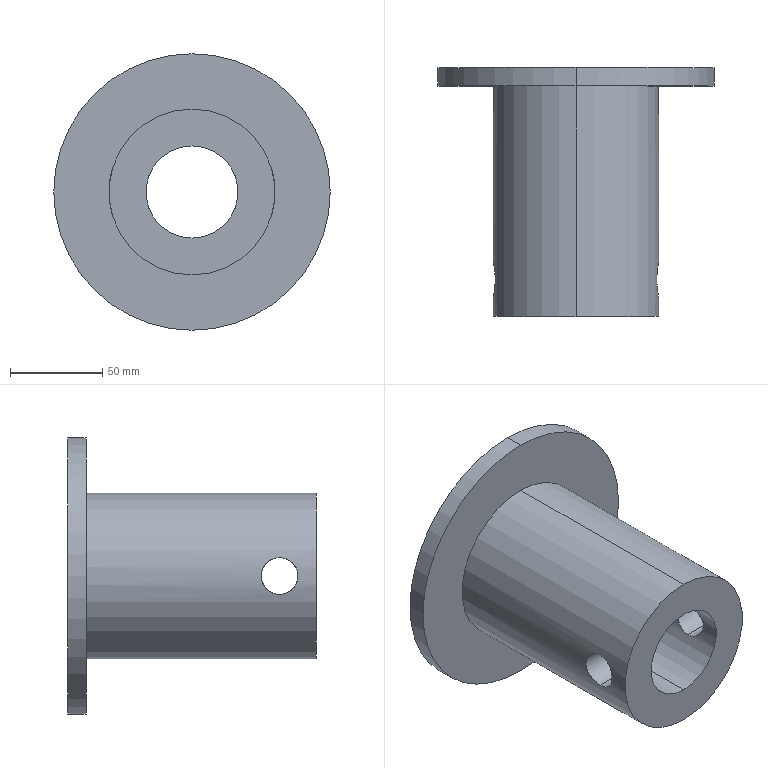Part | SolidWorks | features ICE 2, Extrusion 1 | 1 solid | 13 faces | box 150 x 135 x 150 mm | volume 694147 mm3 | cylinder 10 | plane 3 | commonest cylinder face diameters 20 x4 50 x2 90 x2 150 x2
STEP:
#1=CARTESIAN_POINT('',(-43.875,-105.,10.));
#2=VERTEX_POINT('',#1);
#3=CARTESIAN_POINT('',(-43.875,-105.,-10.));
#4=VERTEX_POINT('',#3);
#5=CARTESIAN_POINT('',(-43.875,-105.,10.));
#6=CARTESIAN_POINT('',(-43.875,-105.654,10.));
#7=CARTESIAN_POINT('',(-43.889,-106.305,9.937));
#8=CARTESIAN_POINT('',(-43.947,-107.602,9.678));
#9=CARTESIAN_POINT('',(-43.989,-108.229,9.487));
#10=CARTESIAN_POINT('',(-44.068,-109.132,9.112));
#11=CARTESIAN_POINT('',(-44.097,-109.427,8.973));
#12=CARTESIAN_POINT('',(-44.158,-110.005,8.663));
#13=CARTESIAN_POINT('',(-44.192,-110.289,8.493));
#14=CARTESIAN_POINT('',(-44.294,-111.104,7.948));
#15=CARTESIAN_POINT('',(-44.367,-111.606,7.536));
#16=CARTESIAN_POINT('',(-44.477,-112.298,6.845));
#17=CARTESIAN_POINT('',(-44.514,-112.519,6.601));
#18=CARTESIAN_POINT('',(-44.586,-112.936,6.094));
#19=CARTESIAN_POINT('',(-44.621,-113.13,5.831));
#20=CARTESIAN_POINT('',(-44.722,-113.673,5.02));
#21=CARTESIAN_POINT('',(-44.784,-113.981,4.447));
#22=CARTESIAN_POINT('',(-44.862,-114.36,3.536));
#23=CARTESIAN_POINT('',(-44.885,-114.472,3.224));
#24=CARTESIAN_POINT('',(-44.926,-114.662,2.598));
#25=CARTESIAN_POINT('',(-44.961,-114.821,1.965));
#26=CARTESIAN_POINT('',(-44.982,-114.918,1.318));
#27=CARTESIAN_POINT('',(-44.996,-114.983,0.6657));
#28=CARTESIAN_POINT('',(-45.,-115.,0.3341));
#29=CARTESIAN_POINT('',(-45.,-115.,-0.6558));
#30=CARTESIAN_POINT('',(-44.986,-114.936,-1.306));
#31=CARTESIAN_POINT('',(-44.93,-114.681,-2.589));
#32=CARTESIAN_POINT('',(-44.888,-114.488,-3.227));
#33=CARTESIAN_POINT('',(-44.785,-113.987,-4.434));
#34=CARTESIAN_POINT('',(-44.724,-113.68,-5.008));
#35=CARTESIAN_POINT('',(-44.622,-113.135,-5.825));
#36=CARTESIAN_POINT('',(-44.587,-112.938,-6.091));
#37=CARTESIAN_POINT('',(-44.515,-112.523,-6.596));
#38=CARTESIAN_POINT('',(-44.478,-112.305,-6.837));
#39=CARTESIAN_POINT('',(-44.405,-111.846,-7.297));
#40=CARTESIAN_POINT('',(-44.369,-111.605,-7.515));
#41=CARTESIAN_POINT('',(-44.296,-111.102,-7.929));
#42=CARTESIAN_POINT('',(-44.261,-110.838,-8.126));
#43=CARTESIAN_POINT('',(-44.158,-110.019,-8.674));
#44=CARTESIAN_POINT('',(-44.095,-109.445,-8.982));
#45=CARTESIAN_POINT('',(-44.017,-108.543,-9.357));
#46=CARTESIAN_POINT('',(-43.993,-108.235,-9.468));
#47=CARTESIAN_POINT('',(-43.951,-107.606,-9.66));
#48=CARTESIAN_POINT('',(-43.933,-107.284,-9.741));
#49=CARTESIAN_POINT('',(-43.89,-106.317,-9.935));
#50=CARTESIAN_POINT('',(-43.875,-105.663,-10.));
#51=CARTESIAN_POINT('',(-43.875,-105.,-10.));
#52=B_SPLINE_CURVE_WITH_KNOTS('',3,(#5,#6,#7,#8,#9,#10,#11,#12,#13,#14,#15,#16,#17,#18,#19,#20,#21,#22,#23,#24,#25,#26,#27,#28,#29,#30,#31,#32,#33,#34,#35,#36,#37,#38,#39,#40,#41,#42,#43,#44,#45,#46,#47,#48,#49,#50,#51),.UNSPECIFIED.,.F.,.F.,(4,2,2,2,2,2,2,2,2,2,1,2,2,2,2,2,2,2,2,2,2,2,2,4),(0.03136,0.03332,0.03528,0.03626,0.03724,0.0392,0.04018,0.04116,0.04312,0.0441,0.04508,0.04606,0.04704,0.049,0.05096,0.05292,0.0539,0.05488,0.05586,0.05684,0.0588,0.05978,0.06076,0.06272),.UNSPECIFIED.);
#53=EDGE_CURVE('',#2,#4,#52,.T.);
#54=ORIENTED_EDGE('',*,*,#53,.F.);
#55=CARTESIAN_POINT('',(-22.913,-105.,10.));
#56=VERTEX_POINT('',#55);
#57=CARTESIAN_POINT('',(-75.,-105.,10.));
#58=DIRECTION('',(1.,0.,0.));
#59=VECTOR('',#58,1000.);
#60=LINE('',#57,#59);
#61=EDGE_CURVE('',#2,#56,#60,.T.);
#62=ORIENTED_EDGE('',*,*,#61,.T.);
#63=CARTESIAN_POINT('',(-22.913,-105.,-10.));
#64=VERTEX_POINT('',#63);
#65=CARTESIAN_POINT('',(-22.913,-105.,10.));
#66=CARTESIAN_POINT('',(-22.913,-105.329,10.));
#67=CARTESIAN_POINT('',(-22.92,-105.658,9.984));
#68=CARTESIAN_POINT('',(-22.948,-106.316,9.918));
#69=CARTESIAN_POINT('',(-22.97,-106.648,9.869));
#70=CARTESIAN_POINT('',(-23.053,-107.619,9.674));
#71=CARTESIAN_POINT('',(-23.134,-108.244,9.482));
#72=CARTESIAN_POINT('',(-23.284,-109.15,9.104));
#73=CARTESIAN_POINT('',(-23.339,-109.449,8.962));
#74=CARTESIAN_POINT('',(-23.456,-110.024,8.652));
#75=CARTESIAN_POINT('',(-23.517,-110.302,8.485));
#76=CARTESIAN_POINT('',(-23.707,-111.108,7.944));
#77=CARTESIAN_POINT('',(-23.843,-111.61,7.532));
#78=CARTESIAN_POINT('',(-24.115,-112.532,6.61));
#79=CARTESIAN_POINT('',(-24.248,-112.942,6.111));
#80=CARTESIAN_POINT('',(-24.432,-113.482,5.306));
#81=CARTESIAN_POINT('',(-24.491,-113.65,5.028));
#82=CARTESIAN_POINT('',(-24.602,-113.96,4.452));
#83=CARTESIAN_POINT('',(-24.655,-114.103,4.153));
#84=CARTESIAN_POINT('',(-24.796,-114.481,3.247));
#85=CARTESIAN_POINT('',(-24.87,-114.672,2.623));
#86=CARTESIAN_POINT('',(-24.947,-114.867,1.656));
#87=CARTESIAN_POINT('',(-24.967,-114.917,1.327));
#88=CARTESIAN_POINT('',(-24.993,-114.983,0.6643));
#89=CARTESIAN_POINT('',(-25.,-115.,0.3339));
#90=CARTESIAN_POINT('',(-25.,-115.,-0.6544));
#91=CARTESIAN_POINT('',(-24.974,-114.936,-1.31));
#92=CARTESIAN_POINT('',(-24.897,-114.741,-2.287));
#93=CARTESIAN_POINT('',(-24.866,-114.659,-2.609));
#94=CARTESIAN_POINT('',(-24.792,-114.467,-3.237));
#95=CARTESIAN_POINT('',(-24.749,-114.357,-3.544));
#96=CARTESIAN_POINT('',(-24.656,-114.106,-4.147));
#97=CARTESIAN_POINT('',(-24.604,-113.965,-4.442));
#98=CARTESIAN_POINT('',(-24.493,-113.656,-5.019));
#99=CARTESIAN_POINT('',(-24.433,-113.486,-5.301));
#100=CARTESIAN_POINT('',(-24.248,-112.942,-6.111));
#101=CARTESIAN_POINT('',(-24.115,-112.532,-6.609));
#102=CARTESIAN_POINT('',(-23.912,-111.845,-7.298));
#103=CARTESIAN_POINT('',(-23.844,-111.602,-7.518));
#104=CARTESIAN_POINT('',(-23.71,-111.1,-7.931));
#105=CARTESIAN_POINT('',(-23.644,-110.841,-8.124));
#106=CARTESIAN_POINT('',(-23.454,-110.036,-8.664));
#107=CARTESIAN_POINT('',(-23.336,-109.466,-8.972));
#108=CARTESIAN_POINT('',(-23.185,-108.554,-9.353));
#109=CARTESIAN_POINT('',(-23.139,-108.244,-9.465));
#110=CARTESIAN_POINT('',(-23.06,-107.617,-9.657));
#111=CARTESIAN_POINT('',(-23.026,-107.299,-9.738));
#112=CARTESIAN_POINT('',(-22.97,-106.655,-9.867));
#113=CARTESIAN_POINT('',(-22.949,-106.329,-9.917));
#114=CARTESIAN_POINT('',(-22.92,-105.669,-9.983));
#115=CARTESIAN_POINT('',(-22.913,-105.334,-10.));
#116=CARTESIAN_POINT('',(-22.913,-105.,-10.));
#117=B_SPLINE_CURVE_WITH_KNOTS('',3,(#65,#66,#67,#68,#69,#70,#71,#72,#73,#74,#75,#76,#77,#78,#79,#80,#81,#82,#83,#84,#85,#86,#87,#88,#89,#90,#91,#92,#93,#94,#95,#96,#97,#98,#99,#100,#101,#102,#103,#104,#105,#106,#107,#108,#109,#110,#111,#112,#113,#114,#115,#116),.UNSPECIFIED.,.F.,.F.,(4,2,2,2,2,2,2,2,2,2,2,2,2,2,2,2,2,2,2,2,2,2,2,2,2,4),(0.0316,0.03258,0.03357,0.03554,0.03653,0.03752,0.03949,0.04146,0.04245,0.04344,0.04541,0.04639,0.04738,0.04935,0.05034,0.05133,0.05231,0.0533,0.05527,0.05626,0.05725,0.05922,0.06021,0.06119,0.06218,0.06317),.UNSPECIFIED.);
#118=EDGE_CURVE('',#56,#64,#117,.T.);
#119=ORIENTED_EDGE('',*,*,#118,.T.);
#120=CARTESIAN_POINT('',(-75.,-105.,-10.));
#121=DIRECTION('',(1.,0.,0.));
#122=VECTOR('',#121,1000.);
#123=LINE('',#120,#122);
#124=EDGE_CURVE('',#4,#64,#123,.T.);
#125=ORIENTED_EDGE('',*,*,#124,.F.);
#126=EDGE_LOOP('',(#54,#62,#119,#125));
#127=FACE_OUTER_BOUND('',#126,.T.);
#128=CARTESIAN_POINT('',(-75.,-105.,0.));
#129=DIRECTION('',(1.,0.,0.));
#130=DIRECTION('',(0.,0.,-1.));
#131=AXIS2_PLACEMENT_3D('',#128,#129,#130);
#132=CYLINDRICAL_SURFACE('',#131,10.);
#133=ADVANCED_FACE('',(#127),#132,.F.);
#134=CARTESIAN_POINT('',(22.913,-105.,-10.));
#135=VERTEX_POINT('',#134);
#136=CARTESIAN_POINT('',(22.913,-105.,10.));
#137=VERTEX_POINT('',#136);
#138=CARTESIAN_POINT('',(22.913,-105.,-10.));
#139=CARTESIAN_POINT('',(22.913,-105.668,-10.));
#140=CARTESIAN_POINT('',(22.942,-106.324,-9.934));
#141=CARTESIAN_POINT('',(23.025,-107.29,-9.74));
#142=CARTESIAN_POINT('',(23.059,-107.608,-9.659));
#143=CARTESIAN_POINT('',(23.139,-108.24,-9.466));
#144=CARTESIAN_POINT('',(23.185,-108.552,-9.354));
#145=CARTESIAN_POINT('',(23.335,-109.457,-8.976));
#146=CARTESIAN_POINT('',(23.452,-110.028,-8.668));
#147=CARTESIAN_POINT('',(23.644,-110.839,-8.125));
#148=CARTESIAN_POINT('',(23.71,-111.103,-7.929));
#149=CARTESIAN_POINT('',(23.844,-111.604,-7.516));
#150=CARTESIAN_POINT('',(23.912,-111.843,-7.299));
#151=CARTESIAN_POINT('',(24.114,-112.528,-6.615));
#152=CARTESIAN_POINT('',(24.247,-112.941,-6.113));
#153=CARTESIAN_POINT('',(24.496,-113.67,-5.026));
#154=CARTESIAN_POINT('',(24.608,-113.977,-4.454));
#155=CARTESIAN_POINT('',(24.748,-114.353,-3.553));
#156=CARTESIAN_POINT('',(24.791,-114.465,-3.245));
#157=CARTESIAN_POINT('',(24.865,-114.658,-2.615));
#158=CARTESIAN_POINT('',(24.897,-114.74,-2.291));
#159=CARTESIAN_POINT('',(24.974,-114.935,-1.32));
#160=CARTESIAN_POINT('',(25.,-115.,-0.6657));
#161=CARTESIAN_POINT('',(25.,-115.,0.3251));
#162=CARTESIAN_POINT('',(24.994,-114.984,0.6588));
#163=CARTESIAN_POINT('',(24.967,-114.918,1.321));
#164=CARTESIAN_POINT('',(24.948,-114.869,1.648));
#165=CARTESIAN_POINT('',(24.871,-114.674,2.615));
#166=CARTESIAN_POINT('',(24.796,-114.483,3.243));
#167=CARTESIAN_POINT('',(24.606,-113.973,4.463));
#168=CARTESIAN_POINT('',(24.494,-113.664,5.036));
#169=CARTESIAN_POINT('',(24.309,-113.122,5.843));
#170=CARTESIAN_POINT('',(24.245,-112.928,6.104));
#171=CARTESIAN_POINT('',(24.112,-112.513,6.608));
#172=CARTESIAN_POINT('',(24.045,-112.293,6.849));
#173=CARTESIAN_POINT('',(23.842,-111.606,7.535));
#174=CARTESIAN_POINT('',(23.707,-111.108,7.945));
#175=CARTESIAN_POINT('',(23.516,-110.298,8.488));
#176=CARTESIAN_POINT('',(23.454,-110.016,8.657));
#177=CARTESIAN_POINT('',(23.337,-109.44,8.966));
#178=CARTESIAN_POINT('',(23.283,-109.146,9.106));
#179=CARTESIAN_POINT('',(23.134,-108.245,9.481));
#180=CARTESIAN_POINT('',(23.053,-107.621,9.673));
#181=CARTESIAN_POINT('',(22.969,-106.644,9.87));
#182=CARTESIAN_POINT('',(22.948,-106.314,9.919));
#183=CARTESIAN_POINT('',(22.92,-105.658,9.984));
#184=CARTESIAN_POINT('',(22.913,-105.329,10.));
#185=CARTESIAN_POINT('',(22.913,-105.,10.));
#186=B_SPLINE_CURVE_WITH_KNOTS('',3,(#138,#139,#140,#141,#142,#143,#144,#145,#146,#147,#148,#149,#150,#151,#152,#153,#154,#155,#156,#157,#158,#159,#160,#161,#162,#163,#164,#165,#166,#167,#168,#169,#170,#171,#172,#173,#174,#175,#176,#177,#178,#179,#180,#181,#182,#183,#184,#185),.UNSPECIFIED.,.F.,.F.,(4,2,2,2,2,2,2,2,2,2,2,2,2,2,2,2,2,2,2,2,2,2,2,4),(0.,0.001975,0.002962,0.00395,0.005924,0.006912,0.007899,0.009874,0.01185,0.01284,0.01382,0.0158,0.01679,0.01777,0.01975,0.02172,0.02271,0.0237,0.02567,0.02666,0.02765,0.02962,0.03061,0.0316),.UNSPECIFIED.);
#187=EDGE_CURVE('',#135,#137,#186,.T.);
#188=ORIENTED_EDGE('',*,*,#187,.T.);
#189=CARTESIAN_POINT('',(43.875,-105.,10.));
#190=VERTEX_POINT('',#189);
#191=CARTESIAN_POINT('',(-75.,-105.,10.));
#192=DIRECTION('',(1.,0.,0.));
#193=VECTOR('',#192,1000.);
#194=LINE('',#191,#193);
#195=EDGE_CURVE('',#137,#190,#194,.T.);
#196=ORIENTED_EDGE('',*,*,#195,.T.);
#197=CARTESIAN_POINT('',(43.875,-105.,-10.));
#198=VERTEX_POINT('',#197);
#199=CARTESIAN_POINT('',(43.875,-105.,-10.));
#200=CARTESIAN_POINT('',(43.875,-105.663,-10.));
#201=CARTESIAN_POINT('',(43.89,-106.314,-9.935));
#202=CARTESIAN_POINT('',(43.933,-107.275,-9.743));
#203=CARTESIAN_POINT('',(43.95,-107.593,-9.664));
#204=CARTESIAN_POINT('',(43.992,-108.222,-9.472));
#205=CARTESIAN_POINT('',(44.016,-108.534,-9.36));
#206=CARTESIAN_POINT('',(44.095,-109.442,-8.983));
#207=CARTESIAN_POINT('',(44.157,-110.015,-8.676));
#208=CARTESIAN_POINT('',(44.26,-110.829,-8.132));
#209=CARTESIAN_POINT('',(44.295,-111.094,-7.935));
#210=CARTESIAN_POINT('',(44.368,-111.601,-7.519));
#211=CARTESIAN_POINT('',(44.405,-111.843,-7.299));
#212=CARTESIAN_POINT('',(44.514,-112.532,-6.61));
#213=CARTESIAN_POINT('',(44.587,-112.945,-6.108));
#214=CARTESIAN_POINT('',(44.689,-113.494,-5.288));
#215=CARTESIAN_POINT('',(44.722,-113.663,-5.005));
#216=CARTESIAN_POINT('',(44.782,-113.971,-4.43));
#217=CARTESIAN_POINT('',(44.811,-114.111,-4.135));
#218=CARTESIAN_POINT('',(44.862,-114.36,-3.534));
#219=CARTESIAN_POINT('',(44.885,-114.471,-3.227));
#220=CARTESIAN_POINT('',(44.926,-114.662,-2.6));
#221=CARTESIAN_POINT('',(44.943,-114.743,-2.278));
#222=CARTESIAN_POINT('',(44.986,-114.936,-1.309));
#223=CARTESIAN_POINT('',(45.,-115.,-0.6585));
#224=CARTESIAN_POINT('',(45.,-115.,0.6506));
#225=CARTESIAN_POINT('',(44.985,-114.935,1.316));
#226=CARTESIAN_POINT('',(44.929,-114.678,2.6));
#227=CARTESIAN_POINT('',(44.888,-114.489,3.224));
#228=CARTESIAN_POINT('',(44.811,-114.111,4.134));
#229=CARTESIAN_POINT('',(44.782,-113.969,4.434));
#230=CARTESIAN_POINT('',(44.721,-113.66,5.011));
#231=CARTESIAN_POINT('',(44.689,-113.492,5.29));
#232=CARTESIAN_POINT('',(44.621,-113.131,5.831));
#233=CARTESIAN_POINT('',(44.586,-112.937,6.092));
#234=CARTESIAN_POINT('',(44.515,-112.523,6.596));
#235=CARTESIAN_POINT('',(44.478,-112.302,6.84));
#236=CARTESIAN_POINT('',(44.367,-111.605,7.536));
#237=CARTESIAN_POINT('',(44.294,-111.103,7.949));
#238=CARTESIAN_POINT('',(44.192,-110.292,8.491));
#239=CARTESIAN_POINT('',(44.159,-110.012,8.66));
#240=CARTESIAN_POINT('',(44.097,-109.432,8.97));
#241=CARTESIAN_POINT('',(44.068,-109.134,9.112));
#242=CARTESIAN_POINT('',(43.989,-108.228,9.487));
#243=CARTESIAN_POINT('',(43.947,-107.604,9.677));
#244=CARTESIAN_POINT('',(43.904,-106.639,9.87));
#245=CARTESIAN_POINT('',(43.893,-106.311,9.919));
#246=CARTESIAN_POINT('',(43.878,-105.654,9.984));
#247=CARTESIAN_POINT('',(43.875,-105.327,10.));
#248=CARTESIAN_POINT('',(43.875,-105.,10.));
#249=B_SPLINE_CURVE_WITH_KNOTS('',3,(#199,#200,#201,#202,#203,#204,#205,#206,#207,#208,#209,#210,#211,#212,#213,#214,#215,#216,#217,#218,#219,#220,#221,#222,#223,#224,#225,#226,#227,#228,#229,#230,#231,#232,#233,#234,#235,#236,#237,#238,#239,#240,#241,#242,#243,#244,#245,#246,#247,#248),.UNSPECIFIED.,.F.,.F.,(4,2,2,2,2,2,2,2,2,2,2,2,2,2,2,2,2,2,2,2,2,2,2,2,4),(0.,0.00196,0.00294,0.00392,0.00588,0.006861,0.007841,0.009801,0.01078,0.01176,0.01274,0.01372,0.01568,0.01764,0.0196,0.02058,0.02156,0.02254,0.02352,0.02548,0.02646,0.02744,0.0294,0.03038,0.03136),.UNSPECIFIED.);
#250=EDGE_CURVE('',#198,#190,#249,.T.);
#251=ORIENTED_EDGE('',*,*,#250,.F.);
#252=CARTESIAN_POINT('',(-75.,-105.,-10.));
#253=DIRECTION('',(1.,0.,0.));
#254=VECTOR('',#253,1000.);
#255=LINE('',#252,#254);
#256=EDGE_CURVE('',#135,#198,#255,.T.);
#257=ORIENTED_EDGE('',*,*,#256,.F.);
#258=EDGE_LOOP('',(#188,#196,#251,#257));
#259=FACE_OUTER_BOUND('',#258,.T.);
#260=CARTESIAN_POINT('',(-75.,-105.,0.));
#261=DIRECTION('',(1.,0.,0.));
#262=DIRECTION('',(0.,0.,-1.));
#263=AXIS2_PLACEMENT_3D('',#260,#261,#262);
#264=CYLINDRICAL_SURFACE('',#263,10.);
#265=ADVANCED_FACE('',(#259),#264,.F.);
#266=ORIENTED_EDGE('',*,*,#250,.T.);
#267=CARTESIAN_POINT('',(43.875,-105.,10.));
#268=CARTESIAN_POINT('',(43.875,-104.346,10.));
#269=CARTESIAN_POINT('',(43.889,-103.695,9.937));
#270=CARTESIAN_POINT('',(43.947,-102.398,9.678));
#271=CARTESIAN_POINT('',(43.989,-101.771,9.487));
#272=CARTESIAN_POINT('',(44.068,-100.868,9.112));
#273=CARTESIAN_POINT('',(44.097,-100.573,8.973));
#274=CARTESIAN_POINT('',(44.158,-99.995,8.663));
#275=CARTESIAN_POINT('',(44.192,-99.711,8.493));
#276=CARTESIAN_POINT('',(44.294,-98.896,7.948));
#277=CARTESIAN_POINT('',(44.367,-98.394,7.536));
#278=CARTESIAN_POINT('',(44.477,-97.702,6.845));
#279=CARTESIAN_POINT('',(44.514,-97.481,6.601));
#280=CARTESIAN_POINT('',(44.586,-97.064,6.094));
#281=CARTESIAN_POINT('',(44.621,-96.87,5.831));
#282=CARTESIAN_POINT('',(44.722,-96.327,5.02));
#283=CARTESIAN_POINT('',(44.784,-96.019,4.447));
#284=CARTESIAN_POINT('',(44.862,-95.64,3.536));
#285=CARTESIAN_POINT('',(44.885,-95.528,3.224));
#286=CARTESIAN_POINT('',(44.926,-95.338,2.598));
#287=CARTESIAN_POINT('',(44.961,-95.179,1.965));
#288=CARTESIAN_POINT('',(44.982,-95.082,1.318));
#289=CARTESIAN_POINT('',(44.996,-95.017,0.6657));
#290=CARTESIAN_POINT('',(45.,-95.,0.3341));
#291=CARTESIAN_POINT('',(45.,-95.,-0.6558));
#292=CARTESIAN_POINT('',(44.986,-95.064,-1.306));
#293=CARTESIAN_POINT('',(44.93,-95.319,-2.589));
#294=CARTESIAN_POINT('',(44.888,-95.512,-3.227));
#295=CARTESIAN_POINT('',(44.785,-96.013,-4.434));
#296=CARTESIAN_POINT('',(44.724,-96.32,-5.008));
#297=CARTESIAN_POINT('',(44.622,-96.865,-5.825));
#298=CARTESIAN_POINT('',(44.587,-97.062,-6.091));
#299=CARTESIAN_POINT('',(44.515,-97.477,-6.596));
#300=CARTESIAN_POINT('',(44.478,-97.695,-6.837));
#301=CARTESIAN_POINT('',(44.405,-98.154,-7.297));
#302=CARTESIAN_POINT('',(44.369,-98.395,-7.515));
#303=CARTESIAN_POINT('',(44.296,-98.898,-7.929));
#304=CARTESIAN_POINT('',(44.261,-99.162,-8.126));
#305=CARTESIAN_POINT('',(44.158,-99.981,-8.674));
#306=CARTESIAN_POINT('',(44.095,-100.555,-8.982));
#307=CARTESIAN_POINT('',(44.017,-101.457,-9.357));
#308=CARTESIAN_POINT('',(43.993,-101.765,-9.468));
#309=CARTESIAN_POINT('',(43.951,-102.394,-9.66));
#310=CARTESIAN_POINT('',(43.933,-102.716,-9.741));
#311=CARTESIAN_POINT('',(43.89,-103.683,-9.935));
#312=CARTESIAN_POINT('',(43.875,-104.337,-10.));
#313=CARTESIAN_POINT('',(43.875,-105.,-10.));
#314=B_SPLINE_CURVE_WITH_KNOTS('',3,(#267,#268,#269,#270,#271,#272,#273,#274,#275,#276,#277,#278,#279,#280,#281,#282,#283,#284,#285,#286,#287,#288,#289,#290,#291,#292,#293,#294,#295,#296,#297,#298,#299,#300,#301,#302,#303,#304,#305,#306,#307,#308,#309,#310,#311,#312,#313),.UNSPECIFIED.,.F.,.F.,(4,2,2,2,2,2,2,2,2,2,1,2,2,2,2,2,2,2,2,2,2,2,2,4),(0.03136,0.03332,0.03528,0.03626,0.03724,0.0392,0.04018,0.04116,0.04312,0.0441,0.04508,0.04606,0.04704,0.049,0.05096,0.05292,0.0539,0.05488,0.05586,0.05684,0.0588,0.05978,0.06076,0.06272),.UNSPECIFIED.);
#315=EDGE_CURVE('',#190,#198,#314,.T.);
#316=ORIENTED_EDGE('',*,*,#315,.T.);
#317=EDGE_LOOP('',(#266,#316));
#318=FACE_BOUND('',#317,.T.);
#319=CARTESIAN_POINT('',(0.,-125.,-45.));
#320=VERTEX_POINT('',#319);
#321=CARTESIAN_POINT('',(0.,-125.,45.));
#322=VERTEX_POINT('',#321);
#323=CARTESIAN_POINT('',(0.,-125.,0.));
#324=DIRECTION('',(0.,-1.,0.));
#325=DIRECTION('',(0.,0.,-1.));
#326=AXIS2_PLACEMENT_3D('',#323,#324,#325);
#327=CIRCLE('',#326,45.);
#328=EDGE_CURVE('',#320,#322,#327,.T.);
#329=ORIENTED_EDGE('',*,*,#328,.F.);
#330=CARTESIAN_POINT('',(0.,0.,-45.));
#331=VERTEX_POINT('',#330);
#332=CARTESIAN_POINT('',(0.,-125.,-45.));
#333=DIRECTION('',(0.,1.,0.));
#334=VECTOR('',#333,1000.);
#335=LINE('',#332,#334);
#336=EDGE_CURVE('',#320,#331,#335,.T.);
#337=ORIENTED_EDGE('',*,*,#336,.T.);
#338=CARTESIAN_POINT('',(0.,0.,45.));
#339=VERTEX_POINT('',#338);
#340=CARTESIAN_POINT('',(0.,0.,0.));
#341=DIRECTION('',(0.,-1.,0.));
#342=DIRECTION('',(0.,0.,1.));
#343=AXIS2_PLACEMENT_3D('',#340,#341,#342);
#344=CIRCLE('',#343,45.);
#345=EDGE_CURVE('',#331,#339,#344,.T.);
#346=ORIENTED_EDGE('',*,*,#345,.T.);
#347=CARTESIAN_POINT('',(0.,-125.,45.));
#348=DIRECTION('',(0.,1.,0.));
#349=VECTOR('',#348,1000.);
#350=LINE('',#347,#349);
#351=EDGE_CURVE('',#322,#339,#350,.T.);
#352=ORIENTED_EDGE('',*,*,#351,.F.);
#353=EDGE_LOOP('',(#329,#337,#346,#352));
#354=FACE_OUTER_BOUND('',#353,.T.);
#355=CARTESIAN_POINT('',(0.,-125.,0.));
#356=DIRECTION('',(0.,1.,0.));
#357=DIRECTION('',(0.,0.,1.));
#358=AXIS2_PLACEMENT_3D('',#355,#356,#357);
#359=CYLINDRICAL_SURFACE('',#358,45.);
#360=ADVANCED_FACE('',(#318,#354),#359,.T.);
#361=CARTESIAN_POINT('',(-22.913,-105.,-10.));
#362=CARTESIAN_POINT('',(-22.913,-104.332,-10.));
#363=CARTESIAN_POINT('',(-22.942,-103.676,-9.934));
#364=CARTESIAN_POINT('',(-23.025,-102.71,-9.74));
#365=CARTESIAN_POINT('',(-23.059,-102.392,-9.659));
#366=CARTESIAN_POINT('',(-23.139,-101.76,-9.466));
#367=CARTESIAN_POINT('',(-23.185,-101.448,-9.354));
#368=CARTESIAN_POINT('',(-23.335,-100.543,-8.976));
#369=CARTESIAN_POINT('',(-23.452,-99.972,-8.668));
#370=CARTESIAN_POINT('',(-23.644,-99.161,-8.125));
#371=CARTESIAN_POINT('',(-23.71,-98.897,-7.929));
#372=CARTESIAN_POINT('',(-23.844,-98.396,-7.516));
#373=CARTESIAN_POINT('',(-23.912,-98.157,-7.299));
#374=CARTESIAN_POINT('',(-24.114,-97.472,-6.615));
#375=CARTESIAN_POINT('',(-24.247,-97.059,-6.113));
#376=CARTESIAN_POINT('',(-24.496,-96.33,-5.026));
#377=CARTESIAN_POINT('',(-24.608,-96.023,-4.454));
#378=CARTESIAN_POINT('',(-24.748,-95.647,-3.553));
#379=CARTESIAN_POINT('',(-24.791,-95.535,-3.245));
#380=CARTESIAN_POINT('',(-24.865,-95.342,-2.615));
#381=CARTESIAN_POINT('',(-24.897,-95.26,-2.291));
#382=CARTESIAN_POINT('',(-24.974,-95.065,-1.32));
#383=CARTESIAN_POINT('',(-25.,-95.,-0.6657));
#384=CARTESIAN_POINT('',(-25.,-95.,0.3251));
#385=CARTESIAN_POINT('',(-24.994,-95.016,0.6588));
#386=CARTESIAN_POINT('',(-24.967,-95.082,1.321));
#387=CARTESIAN_POINT('',(-24.948,-95.131,1.648));
#388=CARTESIAN_POINT('',(-24.871,-95.326,2.615));
#389=CARTESIAN_POINT('',(-24.796,-95.517,3.243));
#390=CARTESIAN_POINT('',(-24.606,-96.027,4.463));
#391=CARTESIAN_POINT('',(-24.494,-96.336,5.036));
#392=CARTESIAN_POINT('',(-24.309,-96.878,5.843));
#393=CARTESIAN_POINT('',(-24.245,-97.072,6.104));
#394=CARTESIAN_POINT('',(-24.112,-97.487,6.608));
#395=CARTESIAN_POINT('',(-24.045,-97.707,6.849));
#396=CARTESIAN_POINT('',(-23.842,-98.394,7.535));
#397=CARTESIAN_POINT('',(-23.707,-98.892,7.945));
#398=CARTESIAN_POINT('',(-23.516,-99.702,8.488));
#399=CARTESIAN_POINT('',(-23.454,-99.984,8.657));
#400=CARTESIAN_POINT('',(-23.337,-100.56,8.966));
#401=CARTESIAN_POINT('',(-23.283,-100.854,9.106));
#402=CARTESIAN_POINT('',(-23.134,-101.755,9.481));
#403=CARTESIAN_POINT('',(-23.053,-102.379,9.673));
#404=CARTESIAN_POINT('',(-22.969,-103.356,9.87));
#405=CARTESIAN_POINT('',(-22.948,-103.686,9.919));
#406=CARTESIAN_POINT('',(-22.92,-104.342,9.984));
#407=CARTESIAN_POINT('',(-22.913,-104.671,10.));
#408=CARTESIAN_POINT('',(-22.913,-105.,10.));
#409=B_SPLINE_CURVE_WITH_KNOTS('',3,(#361,#362,#363,#364,#365,#366,#367,#368,#369,#370,#371,#372,#373,#374,#375,#376,#377,#378,#379,#380,#381,#382,#383,#384,#385,#386,#387,#388,#389,#390,#391,#392,#393,#394,#395,#396,#397,#398,#399,#400,#401,#402,#403,#404,#405,#406,#407,#408),.UNSPECIFIED.,.F.,.F.,(4,2,2,2,2,2,2,2,2,2,2,2,2,2,2,2,2,2,2,2,2,2,2,4),(0.,0.001975,0.002962,0.00395,0.005924,0.006912,0.007899,0.009874,0.01185,0.01284,0.01382,0.0158,0.01679,0.01777,0.01975,0.02172,0.02271,0.0237,0.02567,0.02666,0.02765,0.02962,0.03061,0.0316),.UNSPECIFIED.);
#410=EDGE_CURVE('',#64,#56,#409,.T.);
#411=ORIENTED_EDGE('',*,*,#410,.F.);
#412=ORIENTED_EDGE('',*,*,#118,.F.);
#413=EDGE_LOOP('',(#411,#412));
#414=FACE_BOUND('',#413,.T.);
#415=CARTESIAN_POINT('',(0.,10.,-25.));
#416=VERTEX_POINT('',#415);
#417=CARTESIAN_POINT('',(0.,10.,25.));
#418=VERTEX_POINT('',#417);
#419=CARTESIAN_POINT('',(0.,10.,0.));
#420=DIRECTION('',(0.,1.,0.));
#421=DIRECTION('',(0.,0.,1.));
#422=AXIS2_PLACEMENT_3D('',#419,#420,#421);
#423=CIRCLE('',#422,25.);
#424=EDGE_CURVE('',#416,#418,#423,.T.);
#425=ORIENTED_EDGE('',*,*,#424,.T.);
#426=CARTESIAN_POINT('',(0.,-125.,25.));
#427=VERTEX_POINT('',#426);
#428=CARTESIAN_POINT('',(0.,10.,25.));
#429=DIRECTION('',(0.,-1.,0.));
#430=VECTOR('',#429,1000.);
#431=LINE('',#428,#430);
#432=EDGE_CURVE('',#418,#427,#431,.T.);
#433=ORIENTED_EDGE('',*,*,#432,.T.);
#434=CARTESIAN_POINT('',(0.,-125.,-25.));
#435=VERTEX_POINT('',#434);
#436=CARTESIAN_POINT('',(0.,-125.,0.));
#437=DIRECTION('',(0.,-1.,0.));
#438=DIRECTION('',(0.,0.,-1.));
#439=AXIS2_PLACEMENT_3D('',#436,#437,#438);
#440=CIRCLE('',#439,25.);
#441=EDGE_CURVE('',#427,#435,#440,.T.);
#442=ORIENTED_EDGE('',*,*,#441,.T.);
#443=CARTESIAN_POINT('',(0.,10.,-25.));
#444=DIRECTION('',(0.,-1.,0.));
#445=VECTOR('',#444,1000.);
#446=LINE('',#443,#445);
#447=EDGE_CURVE('',#416,#435,#446,.T.);
#448=ORIENTED_EDGE('',*,*,#447,.F.);
#449=EDGE_LOOP('',(#425,#433,#442,#448));
#450=FACE_OUTER_BOUND('',#449,.T.);
#451=CARTESIAN_POINT('',(0.,10.,0.));
#452=DIRECTION('',(0.,-1.,0.));
#453=DIRECTION('',(0.,0.,-1.));
#454=AXIS2_PLACEMENT_3D('',#451,#452,#453);
#455=CYLINDRICAL_SURFACE('',#454,25.);
#456=ADVANCED_FACE('',(#414,#450),#455,.F.);
#457=CARTESIAN_POINT('',(0.,10.,75.));
#458=VERTEX_POINT('',#457);
#459=CARTESIAN_POINT('',(0.,10.,-75.));
#460=VERTEX_POINT('',#459);
#461=CARTESIAN_POINT('',(0.,10.,0.));
#462=DIRECTION('',(0.,1.,0.));
#463=DIRECTION('',(0.,0.,1.));
#464=AXIS2_PLACEMENT_3D('',#461,#462,#463);
#465=CIRCLE('',#464,75.);
#466=EDGE_CURVE('',#458,#460,#465,.T.);
#467=ORIENTED_EDGE('',*,*,#466,.F.);
#468=CARTESIAN_POINT('',(0.,0.,75.));
#469=VERTEX_POINT('',#468);
#470=CARTESIAN_POINT('',(0.,10.,75.));
#471=DIRECTION('',(0.,-1.,0.));
#472=VECTOR('',#471,1000.);
#473=LINE('',#470,#472);
#474=EDGE_CURVE('',#458,#469,#473,.T.);
#475=ORIENTED_EDGE('',*,*,#474,.T.);
#476=CARTESIAN_POINT('',(0.,0.,-75.));
#477=VERTEX_POINT('',#476);
#478=CARTESIAN_POINT('',(0.,0.,0.));
#479=DIRECTION('',(0.,1.,0.));
#480=DIRECTION('',(0.,0.,1.));
#481=AXIS2_PLACEMENT_3D('',#478,#479,#480);
#482=CIRCLE('',#481,75.);
#483=EDGE_CURVE('',#469,#477,#482,.T.);
#484=ORIENTED_EDGE('',*,*,#483,.T.);
#485=CARTESIAN_POINT('',(0.,10.,-75.));
#486=DIRECTION('',(0.,-1.,0.));
#487=VECTOR('',#486,1000.);
#488=LINE('',#485,#487);
#489=EDGE_CURVE('',#460,#477,#488,.T.);
#490=ORIENTED_EDGE('',*,*,#489,.F.);
#491=EDGE_LOOP('',(#467,#475,#484,#490));
#492=FACE_OUTER_BOUND('',#491,.T.);
#493=CARTESIAN_POINT('',(0.,10.,0.));
#494=DIRECTION('',(0.,-1.,0.));
#495=DIRECTION('',(0.,0.,-1.));
#496=AXIS2_PLACEMENT_3D('',#493,#494,#495);
#497=CYLINDRICAL_SURFACE('',#496,75.);
#498=ADVANCED_FACE('',(#492),#497,.T.);
#499=CARTESIAN_POINT('',(0.,0.,0.));
#500=DIRECTION('',(0.,1.,0.));
#501=DIRECTION('',(0.,0.,1.));
#502=AXIS2_PLACEMENT_3D('',#499,#500,#501);
#503=CIRCLE('',#502,75.);
#504=EDGE_CURVE('',#477,#469,#503,.T.);
#505=ORIENTED_EDGE('',*,*,#504,.F.);
#506=ORIENTED_EDGE('',*,*,#483,.F.);
#507=EDGE_LOOP('',(#505,#506));
#508=FACE_OUTER_BOUND('',#507,.T.);
#509=CARTESIAN_POINT('',(0.,0.,0.));
#510=DIRECTION('',(0.,-1.,0.));
#511=DIRECTION('',(0.,0.,1.));
#512=AXIS2_PLACEMENT_3D('',#509,#510,#511);
#513=CIRCLE('',#512,45.);
#514=EDGE_CURVE('',#339,#331,#513,.T.);
#515=ORIENTED_EDGE('',*,*,#514,.F.);
#516=ORIENTED_EDGE('',*,*,#345,.F.);
#517=EDGE_LOOP('',(#515,#516));
#518=FACE_BOUND('',#517,.T.);
#519=CARTESIAN_POINT('',(0.,0.,0.));
#520=DIRECTION('',(0.,1.,0.));
#521=DIRECTION('',(0.,0.,1.));
#522=AXIS2_PLACEMENT_3D('',#519,#520,#521);
#523=PLANE('',#522);
#524=ADVANCED_FACE('',(#508,#518),#523,.F.);
#525=CARTESIAN_POINT('',(0.,10.,0.));
#526=DIRECTION('',(0.,1.,0.));
#527=DIRECTION('',(0.,0.,1.));
#528=AXIS2_PLACEMENT_3D('',#525,#526,#527);
#529=CIRCLE('',#528,75.);
#530=EDGE_CURVE('',#460,#458,#529,.T.);
#531=ORIENTED_EDGE('',*,*,#530,.T.);
#532=ORIENTED_EDGE('',*,*,#466,.T.);
#533=EDGE_LOOP('',(#531,#532));
#534=FACE_OUTER_BOUND('',#533,.T.);
#535=ORIENTED_EDGE('',*,*,#424,.F.);
#536=CARTESIAN_POINT('',(0.,10.,0.));
#537=DIRECTION('',(0.,1.,0.));
#538=DIRECTION('',(0.,0.,1.));
#539=AXIS2_PLACEMENT_3D('',#536,#537,#538);
#540=CIRCLE('',#539,25.);
#541=EDGE_CURVE('',#418,#416,#540,.T.);
#542=ORIENTED_EDGE('',*,*,#541,.F.);
#543=EDGE_LOOP('',(#535,#542));
#544=FACE_BOUND('',#543,.T.);
#545=CARTESIAN_POINT('',(0.,10.,0.));
#546=DIRECTION('',(0.,1.,0.));
#547=DIRECTION('',(0.,0.,1.));
#548=AXIS2_PLACEMENT_3D('',#545,#546,#547);
#549=PLANE('',#548);
#550=ADVANCED_FACE('',(#534,#544),#549,.T.);
#551=ORIENTED_EDGE('',*,*,#474,.F.);
#552=ORIENTED_EDGE('',*,*,#530,.F.);
#553=ORIENTED_EDGE('',*,*,#489,.T.);
#554=ORIENTED_EDGE('',*,*,#504,.T.);
#555=EDGE_LOOP('',(#551,#552,#553,#554));
#556=FACE_OUTER_BOUND('',#555,.T.);
#557=CARTESIAN_POINT('',(0.,10.,0.));
#558=DIRECTION('',(0.,-1.,0.));
#559=DIRECTION('',(0.,0.,-1.));
#560=AXIS2_PLACEMENT_3D('',#557,#558,#559);
#561=CYLINDRICAL_SURFACE('',#560,75.);
#562=ADVANCED_FACE('',(#556),#561,.T.);
#563=ORIENTED_EDGE('',*,*,#432,.F.);
#564=ORIENTED_EDGE('',*,*,#541,.T.);
#565=ORIENTED_EDGE('',*,*,#447,.T.);
#566=CARTESIAN_POINT('',(0.,-125.,0.));
#567=DIRECTION('',(0.,-1.,0.));
#568=DIRECTION('',(0.,0.,-1.));
#569=AXIS2_PLACEMENT_3D('',#566,#567,#568);
#570=CIRCLE('',#569,25.);
#571=EDGE_CURVE('',#435,#427,#570,.T.);
#572=ORIENTED_EDGE('',*,*,#571,.T.);
#573=EDGE_LOOP('',(#563,#564,#565,#572));
#574=FACE_OUTER_BOUND('',#573,.T.);
#575=ORIENTED_EDGE('',*,*,#187,.F.);
#576=CARTESIAN_POINT('',(22.913,-105.,10.));
#577=CARTESIAN_POINT('',(22.913,-104.671,10.));
#578=CARTESIAN_POINT('',(22.92,-104.342,9.984));
#579=CARTESIAN_POINT('',(22.948,-103.684,9.918));
#580=CARTESIAN_POINT('',(22.97,-103.352,9.869));
#581=CARTESIAN_POINT('',(23.053,-102.381,9.674));
#582=CARTESIAN_POINT('',(23.134,-101.756,9.482));
#583=CARTESIAN_POINT('',(23.284,-100.85,9.104));
#584=CARTESIAN_POINT('',(23.339,-100.551,8.962));
#585=CARTESIAN_POINT('',(23.456,-99.976,8.652));
#586=CARTESIAN_POINT('',(23.517,-99.698,8.485));
#587=CARTESIAN_POINT('',(23.707,-98.892,7.944));
#588=CARTESIAN_POINT('',(23.843,-98.39,7.532));
#589=CARTESIAN_POINT('',(24.115,-97.468,6.61));
#590=CARTESIAN_POINT('',(24.248,-97.058,6.111));
#591=CARTESIAN_POINT('',(24.432,-96.518,5.306));
#592=CARTESIAN_POINT('',(24.491,-96.35,5.028));
#593=CARTESIAN_POINT('',(24.602,-96.04,4.452));
#594=CARTESIAN_POINT('',(24.655,-95.897,4.153));
#595=CARTESIAN_POINT('',(24.796,-95.519,3.247));
#596=CARTESIAN_POINT('',(24.87,-95.328,2.623));
#597=CARTESIAN_POINT('',(24.947,-95.133,1.656));
#598=CARTESIAN_POINT('',(24.967,-95.083,1.327));
#599=CARTESIAN_POINT('',(24.993,-95.017,0.6643));
#600=CARTESIAN_POINT('',(25.,-95.,0.3339));
#601=CARTESIAN_POINT('',(25.,-95.,-0.6544));
#602=CARTESIAN_POINT('',(24.974,-95.064,-1.31));
#603=CARTESIAN_POINT('',(24.897,-95.259,-2.287));
#604=CARTESIAN_POINT('',(24.866,-95.341,-2.609));
#605=CARTESIAN_POINT('',(24.792,-95.533,-3.237));
#606=CARTESIAN_POINT('',(24.749,-95.643,-3.544));
#607=CARTESIAN_POINT('',(24.656,-95.894,-4.147));
#608=CARTESIAN_POINT('',(24.604,-96.035,-4.442));
#609=CARTESIAN_POINT('',(24.493,-96.344,-5.019));
#610=CARTESIAN_POINT('',(24.433,-96.514,-5.301));
#611=CARTESIAN_POINT('',(24.248,-97.058,-6.111));
#612=CARTESIAN_POINT('',(24.115,-97.468,-6.609));
#613=CARTESIAN_POINT('',(23.912,-98.155,-7.298));
#614=CARTESIAN_POINT('',(23.844,-98.398,-7.518));
#615=CARTESIAN_POINT('',(23.71,-98.9,-7.931));
#616=CARTESIAN_POINT('',(23.644,-99.159,-8.124));
#617=CARTESIAN_POINT('',(23.454,-99.964,-8.664));
#618=CARTESIAN_POINT('',(23.336,-100.534,-8.972));
#619=CARTESIAN_POINT('',(23.185,-101.446,-9.353));
#620=CARTESIAN_POINT('',(23.139,-101.756,-9.465));
#621=CARTESIAN_POINT('',(23.06,-102.383,-9.657));
#622=CARTESIAN_POINT('',(23.026,-102.701,-9.738));
#623=CARTESIAN_POINT('',(22.97,-103.345,-9.867));
#624=CARTESIAN_POINT('',(22.949,-103.671,-9.917));
#625=CARTESIAN_POINT('',(22.92,-104.331,-9.983));
#626=CARTESIAN_POINT('',(22.913,-104.666,-10.));
#627=CARTESIAN_POINT('',(22.913,-105.,-10.));
#628=B_SPLINE_CURVE_WITH_KNOTS('',3,(#576,#577,#578,#579,#580,#581,#582,#583,#584,#585,#586,#587,#588,#589,#590,#591,#592,#593,#594,#595,#596,#597,#598,#599,#600,#601,#602,#603,#604,#605,#606,#607,#608,#609,#610,#611,#612,#613,#614,#615,#616,#617,#618,#619,#620,#621,#622,#623,#624,#625,#626,#627),.UNSPECIFIED.,.F.,.F.,(4,2,2,2,2,2,2,2,2,2,2,2,2,2,2,2,2,2,2,2,2,2,2,2,2,4),(0.0316,0.03258,0.03357,0.03554,0.03653,0.03752,0.03949,0.04146,0.04245,0.04344,0.04541,0.04639,0.04738,0.04935,0.05034,0.05133,0.05231,0.0533,0.05527,0.05626,0.05725,0.05922,0.06021,0.06119,0.06218,0.06317),.UNSPECIFIED.);
#629=EDGE_CURVE('',#137,#135,#628,.T.);
#630=ORIENTED_EDGE('',*,*,#629,.F.);
#631=EDGE_LOOP('',(#575,#630));
#632=FACE_BOUND('',#631,.T.);
#633=CARTESIAN_POINT('',(0.,10.,0.));
#634=DIRECTION('',(0.,-1.,0.));
#635=DIRECTION('',(0.,0.,-1.));
#636=AXIS2_PLACEMENT_3D('',#633,#634,#635);
#637=CYLINDRICAL_SURFACE('',#636,25.);
#638=ADVANCED_FACE('',(#574,#632),#637,.F.);
#639=CARTESIAN_POINT('',(0.,-125.,0.));
#640=DIRECTION('',(0.,-1.,0.));
#641=DIRECTION('',(0.,0.,-1.));
#642=AXIS2_PLACEMENT_3D('',#639,#640,#641);
#643=CIRCLE('',#642,45.);
#644=EDGE_CURVE('',#322,#320,#643,.T.);
#645=ORIENTED_EDGE('',*,*,#644,.T.);
#646=ORIENTED_EDGE('',*,*,#328,.T.);
#647=EDGE_LOOP('',(#645,#646));
#648=FACE_OUTER_BOUND('',#647,.T.);
#649=ORIENTED_EDGE('',*,*,#571,.F.);
#650=ORIENTED_EDGE('',*,*,#441,.F.);
#651=EDGE_LOOP('',(#649,#650));
#652=FACE_BOUND('',#651,.T.);
#653=CARTESIAN_POINT('',(0.,-125.,0.));
#654=DIRECTION('',(0.,-1.,0.));
#655=DIRECTION('',(0.,0.,-1.));
#656=AXIS2_PLACEMENT_3D('',#653,#654,#655);
#657=PLANE('',#656);
#658=ADVANCED_FACE('',(#648,#652),#657,.T.);
#659=ORIENTED_EDGE('',*,*,#336,.F.);
#660=ORIENTED_EDGE('',*,*,#644,.F.);
#661=ORIENTED_EDGE('',*,*,#351,.T.);
#662=ORIENTED_EDGE('',*,*,#514,.T.);
#663=EDGE_LOOP('',(#659,#660,#661,#662));
#664=FACE_OUTER_BOUND('',#663,.T.);
#665=CARTESIAN_POINT('',(-43.875,-105.,-10.));
#666=CARTESIAN_POINT('',(-43.875,-104.337,-10.));
#667=CARTESIAN_POINT('',(-43.89,-103.686,-9.935));
#668=CARTESIAN_POINT('',(-43.933,-102.725,-9.743));
#669=CARTESIAN_POINT('',(-43.95,-102.407,-9.664));
#670=CARTESIAN_POINT('',(-43.992,-101.778,-9.472));
#671=CARTESIAN_POINT('',(-44.016,-101.466,-9.36));
#672=CARTESIAN_POINT('',(-44.095,-100.558,-8.983));
#673=CARTESIAN_POINT('',(-44.157,-99.985,-8.676));
#674=CARTESIAN_POINT('',(-44.26,-99.171,-8.132));
#675=CARTESIAN_POINT('',(-44.295,-98.906,-7.935));
#676=CARTESIAN_POINT('',(-44.368,-98.399,-7.519));
#677=CARTESIAN_POINT('',(-44.405,-98.157,-7.299));
#678=CARTESIAN_POINT('',(-44.514,-97.468,-6.61));
#679=CARTESIAN_POINT('',(-44.587,-97.055,-6.108));
#680=CARTESIAN_POINT('',(-44.689,-96.506,-5.288));
#681=CARTESIAN_POINT('',(-44.722,-96.337,-5.005));
#682=CARTESIAN_POINT('',(-44.782,-96.029,-4.43));
#683=CARTESIAN_POINT('',(-44.811,-95.889,-4.135));
#684=CARTESIAN_POINT('',(-44.862,-95.64,-3.534));
#685=CARTESIAN_POINT('',(-44.885,-95.529,-3.227));
#686=CARTESIAN_POINT('',(-44.926,-95.338,-2.6));
#687=CARTESIAN_POINT('',(-44.943,-95.257,-2.278));
#688=CARTESIAN_POINT('',(-44.986,-95.064,-1.309));
#689=CARTESIAN_POINT('',(-45.,-95.,-0.6585));
#690=CARTESIAN_POINT('',(-45.,-95.,0.6506));
#691=CARTESIAN_POINT('',(-44.985,-95.065,1.316));
#692=CARTESIAN_POINT('',(-44.929,-95.322,2.6));
#693=CARTESIAN_POINT('',(-44.888,-95.511,3.224));
#694=CARTESIAN_POINT('',(-44.811,-95.889,4.134));
#695=CARTESIAN_POINT('',(-44.782,-96.031,4.434));
#696=CARTESIAN_POINT('',(-44.721,-96.34,5.011));
#697=CARTESIAN_POINT('',(-44.689,-96.508,5.29));
#698=CARTESIAN_POINT('',(-44.621,-96.869,5.831));
#699=CARTESIAN_POINT('',(-44.586,-97.063,6.092));
#700=CARTESIAN_POINT('',(-44.515,-97.477,6.596));
#701=CARTESIAN_POINT('',(-44.478,-97.698,6.84));
#702=CARTESIAN_POINT('',(-44.367,-98.395,7.536));
#703=CARTESIAN_POINT('',(-44.294,-98.897,7.949));
#704=CARTESIAN_POINT('',(-44.192,-99.708,8.491));
#705=CARTESIAN_POINT('',(-44.159,-99.988,8.66));
#706=CARTESIAN_POINT('',(-44.097,-100.568,8.97));
#707=CARTESIAN_POINT('',(-44.068,-100.866,9.112));
#708=CARTESIAN_POINT('',(-43.989,-101.772,9.487));
#709=CARTESIAN_POINT('',(-43.947,-102.396,9.677));
#710=CARTESIAN_POINT('',(-43.904,-103.361,9.87));
#711=CARTESIAN_POINT('',(-43.893,-103.689,9.919));
#712=CARTESIAN_POINT('',(-43.878,-104.346,9.984));
#713=CARTESIAN_POINT('',(-43.875,-104.673,10.));
#714=CARTESIAN_POINT('',(-43.875,-105.,10.));
#715=B_SPLINE_CURVE_WITH_KNOTS('',3,(#665,#666,#667,#668,#669,#670,#671,#672,#673,#674,#675,#676,#677,#678,#679,#680,#681,#682,#683,#684,#685,#686,#687,#688,#689,#690,#691,#692,#693,#694,#695,#696,#697,#698,#699,#700,#701,#702,#703,#704,#705,#706,#707,#708,#709,#710,#711,#712,#713,#714),.UNSPECIFIED.,.F.,.F.,(4,2,2,2,2,2,2,2,2,2,2,2,2,2,2,2,2,2,2,2,2,2,2,2,4),(0.,0.00196,0.00294,0.00392,0.00588,0.006861,0.007841,0.009801,0.01078,0.01176,0.01274,0.01372,0.01568,0.01764,0.0196,0.02058,0.02156,0.02254,0.02352,0.02548,0.02646,0.02744,0.0294,0.03038,0.03136),.UNSPECIFIED.);
#716=EDGE_CURVE('',#4,#2,#715,.T.);
#717=ORIENTED_EDGE('',*,*,#716,.T.);
#718=ORIENTED_EDGE('',*,*,#53,.T.);
#719=EDGE_LOOP('',(#717,#718));
#720=FACE_BOUND('',#719,.T.);
#721=CARTESIAN_POINT('',(0.,-125.,0.));
#722=DIRECTION('',(0.,1.,0.));
#723=DIRECTION('',(0.,0.,1.));
#724=AXIS2_PLACEMENT_3D('',#721,#722,#723);
#725=CYLINDRICAL_SURFACE('',#724,45.);
#726=ADVANCED_FACE('',(#664,#720),#725,.T.);
#727=ORIENTED_EDGE('',*,*,#195,.F.);
#728=ORIENTED_EDGE('',*,*,#629,.T.);
#729=ORIENTED_EDGE('',*,*,#256,.T.);
#730=ORIENTED_EDGE('',*,*,#315,.F.);
#731=EDGE_LOOP('',(#727,#728,#729,#730));
#732=FACE_OUTER_BOUND('',#731,.T.);
#733=CARTESIAN_POINT('',(-75.,-105.,0.));
#734=DIRECTION('',(1.,0.,0.));
#735=DIRECTION('',(0.,0.,-1.));
#736=AXIS2_PLACEMENT_3D('',#733,#734,#735);
#737=CYLINDRICAL_SURFACE('',#736,10.);
#738=ADVANCED_FACE('',(#732),#737,.F.);
#739=ORIENTED_EDGE('',*,*,#61,.F.);
#740=ORIENTED_EDGE('',*,*,#716,.F.);
#741=ORIENTED_EDGE('',*,*,#124,.T.);
#742=ORIENTED_EDGE('',*,*,#410,.T.);
#743=EDGE_LOOP('',(#739,#740,#741,#742));
#744=FACE_OUTER_BOUND('',#743,.T.);
#745=CARTESIAN_POINT('',(-75.,-105.,0.));
#746=DIRECTION('',(1.,0.,0.));
#747=DIRECTION('',(0.,0.,-1.));
#748=AXIS2_PLACEMENT_3D('',#745,#746,#747);
#749=CYLINDRICAL_SURFACE('',#748,10.);
#750=ADVANCED_FACE('',(#744),#749,.F.);
#751=CLOSED_SHELL('',(#133,#265,#360,#456,#498,#524,#550,#562,#638,#658,#726,#738,#750));
#752=MANIFOLD_SOLID_BREP('',#751);
#753=CARTESIAN_POINT('',(0.,0.,0.));
#754=DIRECTION('',(0.,0.,1.));
#755=DIRECTION('',(1.,0.,0.));
#756=AXIS2_PLACEMENT_3D('',#753,#754,#755);
#757=(LENGTH_UNIT()NAMED_UNIT(*)SI_UNIT(.MILLI.,.METRE.));
#758=UNCERTAINTY_MEASURE_WITH_UNIT(LENGTH_MEASURE(0.00001),#757,'','');
#759=(NAMED_UNIT(*)PLANE_ANGLE_UNIT()SI_UNIT($,.RADIAN.));
#760=(NAMED_UNIT(*)SI_UNIT($,.STERADIAN.)SOLID_ANGLE_UNIT());
#761=(GEOMETRIC_REPRESENTATION_CONTEXT(3)GLOBAL_UNCERTAINTY_ASSIGNED_CONTEXT((#758))GLOBAL_UNIT_ASSIGNED_CONTEXT((#757,#759,#760))REPRESENTATION_CONTEXT('',''));
#762=ADVANCED_BREP_SHAPE_REPRESENTATION('',(#752,#756),#761);